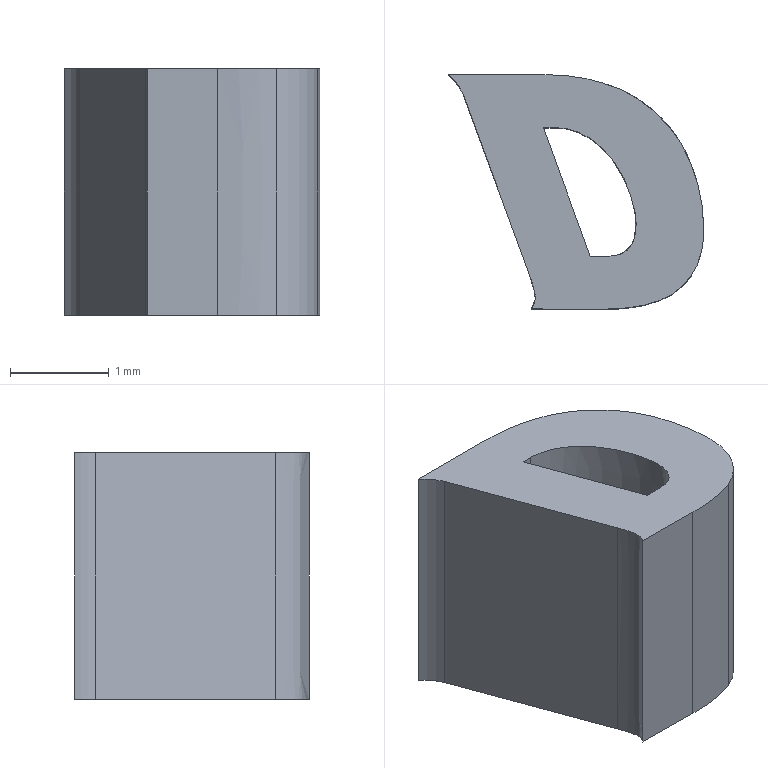Part | STEP file | lll_id1118_x_t | 1 solid | 17 faces | box 2.599 x 2.384 x 2.5 mm | volume 9.059 mm3 | plane 8 | other 6 | cylinder 3 | commonest cylinder face diameters 1.036 x1 1.35 x1 2.111 x1
STEP:
#1=CARTESIAN_POINT('',(392.289,-127.34,2.35));
#2=VERTEX_POINT('',#1);
#3=CARTESIAN_POINT('',(392.454,-127.34,2.35));
#4=VERTEX_POINT('',#3);
#5=CARTESIAN_POINT('',(392.289,-127.34,2.35));
#6=DIRECTION('',(1.,0.,0.));
#7=VECTOR('',#6,1.);
#8=LINE('',#5,#7);
#9=EDGE_CURVE('',#2,#4,#8,.T.);
#10=ORIENTED_EDGE('',*,*,#9,.T.);
#11=CARTESIAN_POINT('',(392.454,-127.34,-0.15));
#12=VERTEX_POINT('',#11);
#13=CARTESIAN_POINT('',(392.454,-127.34,-0.15));
#14=DIRECTION('',(0.,0.,1.));
#15=VECTOR('',#14,1.);
#16=LINE('',#13,#15);
#17=EDGE_CURVE('',#12,#4,#16,.T.);
#18=ORIENTED_EDGE('',*,*,#17,.F.);
#19=CARTESIAN_POINT('',(392.289,-127.34,-0.15));
#20=VERTEX_POINT('',#19);
#21=CARTESIAN_POINT('',(392.289,-127.34,-0.15));
#22=DIRECTION('',(1.,0.,0.));
#23=VECTOR('',#22,1.);
#24=LINE('',#21,#23);
#25=EDGE_CURVE('',#20,#12,#24,.T.);
#26=ORIENTED_EDGE('',*,*,#25,.F.);
#27=CARTESIAN_POINT('',(392.289,-127.34,-0.15));
#28=DIRECTION('',(0.,0.,1.));
#29=VECTOR('',#28,1.);
#30=LINE('',#27,#29);
#31=EDGE_CURVE('',#20,#2,#30,.T.);
#32=ORIENTED_EDGE('',*,*,#31,.T.);
#33=EDGE_LOOP('',(#10,#18,#26,#32));
#34=FACE_OUTER_BOUND('',#33,.T.);
#35=CARTESIAN_POINT('',(392.289,-127.34,-0.15));
#36=DIRECTION('',(0.,-1.,0.));
#37=DIRECTION('',(0.,0.,-1.));
#38=AXIS2_PLACEMENT_3D('',#35,#36,#37);
#39=PLANE('',#38);
#40=ADVANCED_FACE('',(#34),#39,.F.);
#41=CARTESIAN_POINT('',(392.629,-127.301,2.35));
#42=VERTEX_POINT('',#41);
#43=CARTESIAN_POINT('',(392.454,-127.34,2.35));
#44=CARTESIAN_POINT('',(392.485,-127.34,2.35));
#45=CARTESIAN_POINT('',(392.515,-127.337,2.35));
#46=CARTESIAN_POINT('',(392.574,-127.326,2.35));
#47=CARTESIAN_POINT('',(392.603,-127.316,2.35));
#48=CARTESIAN_POINT('',(392.629,-127.301,2.35));
#49=(BOUNDED_CURVE()B_SPLINE_CURVE(3,(#43,#44,#45,#46,#47,#48),.UNSPECIFIED.,.F.,.F.)B_SPLINE_CURVE_WITH_KNOTS((4,2,4),(0.,0.5014,1.),.UNSPECIFIED.)CURVE()GEOMETRIC_REPRESENTATION_ITEM()RATIONAL_B_SPLINE_CURVE((0.5011,0.4996,0.4996,0.4968,0.4968,0.5011))REPRESENTATION_ITEM(''));
#50=EDGE_CURVE('',#4,#42,#49,.T.);
#51=ORIENTED_EDGE('',*,*,#50,.T.);
#52=CARTESIAN_POINT('',(392.629,-127.301,-0.15));
#53=VERTEX_POINT('',#52);
#54=CARTESIAN_POINT('',(392.629,-127.301,-0.15));
#55=DIRECTION('',(0.,0.,1.));
#56=VECTOR('',#55,1.);
#57=LINE('',#54,#56);
#58=EDGE_CURVE('',#53,#42,#57,.T.);
#59=ORIENTED_EDGE('',*,*,#58,.F.);
#60=CARTESIAN_POINT('',(392.454,-127.34,-0.15));
#61=CARTESIAN_POINT('',(392.485,-127.34,-0.15));
#62=CARTESIAN_POINT('',(392.515,-127.337,-0.15));
#63=CARTESIAN_POINT('',(392.574,-127.326,-0.15));
#64=CARTESIAN_POINT('',(392.603,-127.316,-0.15));
#65=CARTESIAN_POINT('',(392.629,-127.301,-0.15));
#66=(BOUNDED_CURVE()B_SPLINE_CURVE(3,(#60,#61,#62,#63,#64,#65),.UNSPECIFIED.,.F.,.F.)B_SPLINE_CURVE_WITH_KNOTS((4,2,4),(0.,0.5014,1.),.UNSPECIFIED.)CURVE()GEOMETRIC_REPRESENTATION_ITEM()RATIONAL_B_SPLINE_CURVE((0.5011,0.4996,0.4996,0.4968,0.4968,0.5011))REPRESENTATION_ITEM(''));
#67=EDGE_CURVE('',#12,#53,#66,.T.);
#68=ORIENTED_EDGE('',*,*,#67,.F.);
#69=ORIENTED_EDGE('',*,*,#17,.T.);
#70=EDGE_LOOP('',(#51,#59,#68,#69));
#71=FACE_OUTER_BOUND('',#70,.T.);
#72=CARTESIAN_POINT('',(392.454,-127.34,-0.15));
#73=CARTESIAN_POINT('',(392.485,-127.34,-0.15));
#74=CARTESIAN_POINT('',(392.515,-127.337,-0.15));
#75=CARTESIAN_POINT('',(392.574,-127.326,-0.15));
#76=CARTESIAN_POINT('',(392.603,-127.316,-0.15));
#77=CARTESIAN_POINT('',(392.629,-127.301,-0.15));
#78=(BOUNDED_CURVE()B_SPLINE_CURVE(3,(#72,#73,#74,#75,#76,#77),.UNSPECIFIED.,.F.,.F.)B_SPLINE_CURVE_WITH_KNOTS((4,2,4),(0.,0.5014,1.),.UNSPECIFIED.)CURVE()GEOMETRIC_REPRESENTATION_ITEM()RATIONAL_B_SPLINE_CURVE((0.5011,0.4996,0.4996,0.4968,0.4968,0.5011))REPRESENTATION_ITEM(''));
#79=DIRECTION('',(0.,0.,1.));
#80=VECTOR('',#79,1.);
#81=SURFACE_OF_LINEAR_EXTRUSION('',#78,#80);
#82=ADVANCED_FACE('',(#71),#81,.F.);
#83=CARTESIAN_POINT('',(391.925,-126.033,2.35));
#84=VERTEX_POINT('',#83);
#85=CARTESIAN_POINT('',(392.629,-127.301,2.35));
#86=CARTESIAN_POINT('',(392.664,-127.281,2.35));
#87=CARTESIAN_POINT('',(392.693,-127.252,2.35));
#88=CARTESIAN_POINT('',(392.724,-127.194,2.35));
#89=CARTESIAN_POINT('',(392.733,-127.17,2.35));
#90=CARTESIAN_POINT('',(392.748,-127.112,2.35));
#91=CARTESIAN_POINT('',(392.753,-127.077,2.35));
#92=CARTESIAN_POINT('',(392.755,-127.012,2.35));
#93=CARTESIAN_POINT('',(392.754,-126.982,2.35));
#94=CARTESIAN_POINT('',(392.746,-126.903,2.35));
#95=CARTESIAN_POINT('',(392.737,-126.854,2.35));
#96=CARTESIAN_POINT('',(392.689,-126.67,2.35));
#97=CARTESIAN_POINT('',(392.635,-126.542,2.35));
#98=CARTESIAN_POINT('',(392.512,-126.348,2.35));
#99=CARTESIAN_POINT('',(392.454,-126.279,2.35));
#100=CARTESIAN_POINT('',(392.321,-126.158,2.35));
#101=CARTESIAN_POINT('',(392.244,-126.11,2.35));
#102=CARTESIAN_POINT('',(392.085,-126.047,2.35));
#103=CARTESIAN_POINT('',(392.006,-126.033,2.35));
#104=CARTESIAN_POINT('',(391.925,-126.033,2.35));
#105=(BOUNDED_CURVE()B_SPLINE_CURVE(3,(#85,#86,#87,#88,#89,#90,#91,#92,#93,#94,#95,#96,#97,#98,#99,#100,#101,#102,#103,#104),.UNSPECIFIED.,.F.,.F.)B_SPLINE_CURVE_WITH_KNOTS((4,2,2,2,2,2,2,2,2,4),(0.,0.07173,0.1159,0.1772,0.2294,0.3163,0.5576,0.7116,0.8649,1.),.UNSPECIFIED.)CURVE()GEOMETRIC_REPRESENTATION_ITEM()RATIONAL_B_SPLINE_CURVE((0.5011,0.4882,0.4882,0.4987,0.4987,0.499,0.499,0.5004,0.5004,0.5001,0.5001,0.497,0.497,0.4981,0.4981,0.4957,0.4957,0.4952,0.4952,0.5011))REPRESENTATION_ITEM(''));
#106=EDGE_CURVE('',#42,#84,#105,.T.);
#107=ORIENTED_EDGE('',*,*,#106,.T.);
#108=CARTESIAN_POINT('',(391.925,-126.033,-0.15));
#109=VERTEX_POINT('',#108);
#110=CARTESIAN_POINT('',(391.925,-126.033,-0.15));
#111=DIRECTION('',(0.,0.,1.));
#112=VECTOR('',#111,1.);
#113=LINE('',#110,#112);
#114=EDGE_CURVE('',#109,#84,#113,.T.);
#115=ORIENTED_EDGE('',*,*,#114,.F.);
#116=CARTESIAN_POINT('',(392.629,-127.301,-0.15));
#117=CARTESIAN_POINT('',(392.664,-127.281,-0.15));
#118=CARTESIAN_POINT('',(392.693,-127.252,-0.15));
#119=CARTESIAN_POINT('',(392.724,-127.194,-0.15));
#120=CARTESIAN_POINT('',(392.733,-127.17,-0.15));
#121=CARTESIAN_POINT('',(392.748,-127.112,-0.15));
#122=CARTESIAN_POINT('',(392.753,-127.077,-0.15));
#123=CARTESIAN_POINT('',(392.755,-127.012,-0.15));
#124=CARTESIAN_POINT('',(392.754,-126.982,-0.15));
#125=CARTESIAN_POINT('',(392.746,-126.903,-0.15));
#126=CARTESIAN_POINT('',(392.737,-126.854,-0.15));
#127=CARTESIAN_POINT('',(392.689,-126.67,-0.15));
#128=CARTESIAN_POINT('',(392.635,-126.542,-0.15));
#129=CARTESIAN_POINT('',(392.512,-126.348,-0.15));
#130=CARTESIAN_POINT('',(392.454,-126.279,-0.15));
#131=CARTESIAN_POINT('',(392.321,-126.158,-0.15));
#132=CARTESIAN_POINT('',(392.244,-126.11,-0.15));
#133=CARTESIAN_POINT('',(392.085,-126.047,-0.15));
#134=CARTESIAN_POINT('',(392.006,-126.033,-0.15));
#135=CARTESIAN_POINT('',(391.925,-126.033,-0.15));
#136=(BOUNDED_CURVE()B_SPLINE_CURVE(3,(#116,#117,#118,#119,#120,#121,#122,#123,#124,#125,#126,#127,#128,#129,#130,#131,#132,#133,#134,#135),.UNSPECIFIED.,.F.,.F.)B_SPLINE_CURVE_WITH_KNOTS((4,2,2,2,2,2,2,2,2,4),(0.,0.07173,0.1159,0.1772,0.2294,0.3163,0.5576,0.7116,0.8649,1.),.UNSPECIFIED.)CURVE()GEOMETRIC_REPRESENTATION_ITEM()RATIONAL_B_SPLINE_CURVE((0.5011,0.4882,0.4882,0.4987,0.4987,0.499,0.499,0.5004,0.5004,0.5001,0.5001,0.497,0.497,0.4981,0.4981,0.4957,0.4957,0.4952,0.4952,0.5011))REPRESENTATION_ITEM(''));
#137=EDGE_CURVE('',#53,#109,#136,.T.);
#138=ORIENTED_EDGE('',*,*,#137,.F.);
#139=ORIENTED_EDGE('',*,*,#58,.T.);
#140=EDGE_LOOP('',(#107,#115,#138,#139));
#141=FACE_OUTER_BOUND('',#140,.T.);
#142=CARTESIAN_POINT('',(392.629,-127.301,-0.15));
#143=CARTESIAN_POINT('',(392.664,-127.281,-0.15));
#144=CARTESIAN_POINT('',(392.693,-127.252,-0.15));
#145=CARTESIAN_POINT('',(392.724,-127.194,-0.15));
#146=CARTESIAN_POINT('',(392.733,-127.17,-0.15));
#147=CARTESIAN_POINT('',(392.748,-127.112,-0.15));
#148=CARTESIAN_POINT('',(392.753,-127.077,-0.15));
#149=CARTESIAN_POINT('',(392.755,-127.012,-0.15));
#150=CARTESIAN_POINT('',(392.754,-126.982,-0.15));
#151=CARTESIAN_POINT('',(392.746,-126.903,-0.15));
#152=CARTESIAN_POINT('',(392.737,-126.854,-0.15));
#153=CARTESIAN_POINT('',(392.689,-126.67,-0.15));
#154=CARTESIAN_POINT('',(392.635,-126.542,-0.15));
#155=CARTESIAN_POINT('',(392.512,-126.348,-0.15));
#156=CARTESIAN_POINT('',(392.454,-126.279,-0.15));
#157=CARTESIAN_POINT('',(392.321,-126.158,-0.15));
#158=CARTESIAN_POINT('',(392.244,-126.11,-0.15));
#159=CARTESIAN_POINT('',(392.085,-126.047,-0.15));
#160=CARTESIAN_POINT('',(392.006,-126.033,-0.15));
#161=CARTESIAN_POINT('',(391.925,-126.033,-0.15));
#162=(BOUNDED_CURVE()B_SPLINE_CURVE(3,(#142,#143,#144,#145,#146,#147,#148,#149,#150,#151,#152,#153,#154,#155,#156,#157,#158,#159,#160,#161),.UNSPECIFIED.,.F.,.F.)B_SPLINE_CURVE_WITH_KNOTS((4,2,2,2,2,2,2,2,2,4),(0.,0.07173,0.1159,0.1772,0.2294,0.3163,0.5576,0.7116,0.8649,1.),.UNSPECIFIED.)CURVE()GEOMETRIC_REPRESENTATION_ITEM()RATIONAL_B_SPLINE_CURVE((0.5011,0.4882,0.4882,0.4987,0.4987,0.499,0.499,0.5004,0.5004,0.5001,0.5001,0.497,0.497,0.4981,0.4981,0.4957,0.4957,0.4952,0.4952,0.5011))REPRESENTATION_ITEM(''));
#163=DIRECTION('',(0.,0.,1.));
#164=VECTOR('',#163,1.);
#165=SURFACE_OF_LINEAR_EXTRUSION('',#162,#164);
#166=ADVANCED_FACE('',(#141),#165,.F.);
#167=CARTESIAN_POINT('',(391.814,-126.033,2.35));
#168=VERTEX_POINT('',#167);
#169=CARTESIAN_POINT('',(391.925,-126.033,2.35));
#170=DIRECTION('',(-1.,0.,0.));
#171=VECTOR('',#170,1.);
#172=LINE('',#169,#171);
#173=EDGE_CURVE('',#84,#168,#172,.T.);
#174=ORIENTED_EDGE('',*,*,#173,.T.);
#175=CARTESIAN_POINT('',(391.814,-126.033,-0.15));
#176=VERTEX_POINT('',#175);
#177=CARTESIAN_POINT('',(391.814,-126.033,-0.15));
#178=DIRECTION('',(0.,0.,1.));
#179=VECTOR('',#178,1.);
#180=LINE('',#177,#179);
#181=EDGE_CURVE('',#176,#168,#180,.T.);
#182=ORIENTED_EDGE('',*,*,#181,.F.);
#183=CARTESIAN_POINT('',(391.925,-126.033,-0.15));
#184=DIRECTION('',(-1.,0.,0.));
#185=VECTOR('',#184,1.);
#186=LINE('',#183,#185);
#187=EDGE_CURVE('',#109,#176,#186,.T.);
#188=ORIENTED_EDGE('',*,*,#187,.F.);
#189=ORIENTED_EDGE('',*,*,#114,.T.);
#190=EDGE_LOOP('',(#174,#182,#188,#189));
#191=FACE_OUTER_BOUND('',#190,.T.);
#192=CARTESIAN_POINT('',(391.925,-126.033,-0.15));
#193=DIRECTION('',(0.,1.,0.));
#194=DIRECTION('',(0.,0.,1.));
#195=AXIS2_PLACEMENT_3D('',#192,#193,#194);
#196=PLANE('',#195);
#197=ADVANCED_FACE('',(#191),#196,.F.);
#198=CARTESIAN_POINT('',(391.787,-125.492,2.35));
#199=VERTEX_POINT('',#198);
#200=CARTESIAN_POINT('',(392.416,-125.579,2.35));
#201=VERTEX_POINT('',#200);
#202=CARTESIAN_POINT('',(391.787,-125.492,2.35));
#203=CARTESIAN_POINT('',(391.894,-125.492,2.35));
#204=CARTESIAN_POINT('',(392.,-125.499,2.35));
#205=CARTESIAN_POINT('',(392.211,-125.526,2.35));
#206=CARTESIAN_POINT('',(392.315,-125.548,2.35));
#207=CARTESIAN_POINT('',(392.416,-125.579,2.35));
#208=(BOUNDED_CURVE()B_SPLINE_CURVE(3,(#202,#203,#204,#205,#206,#207),.UNSPECIFIED.,.F.,.F.)B_SPLINE_CURVE_WITH_KNOTS((4,2,4),(0.,0.5009,1.),.UNSPECIFIED.)CURVE()GEOMETRIC_REPRESENTATION_ITEM()RATIONAL_B_SPLINE_CURVE((0.5005,0.4998,0.4998,0.4993,0.4993,0.5005))REPRESENTATION_ITEM(''));
#209=EDGE_CURVE('',#199,#201,#208,.T.);
#210=ORIENTED_EDGE('',*,*,#209,.T.);
#211=CARTESIAN_POINT('',(392.416,-125.579,-0.15));
#212=VERTEX_POINT('',#211);
#213=CARTESIAN_POINT('',(392.416,-125.579,-0.15));
#214=DIRECTION('',(0.,0.,1.));
#215=VECTOR('',#214,1.);
#216=LINE('',#213,#215);
#217=EDGE_CURVE('',#212,#201,#216,.T.);
#218=ORIENTED_EDGE('',*,*,#217,.F.);
#219=CARTESIAN_POINT('',(391.787,-125.492,-0.15));
#220=VERTEX_POINT('',#219);
#221=CARTESIAN_POINT('',(391.787,-125.492,-0.15));
#222=CARTESIAN_POINT('',(391.894,-125.492,-0.15));
#223=CARTESIAN_POINT('',(392.,-125.499,-0.15));
#224=CARTESIAN_POINT('',(392.211,-125.526,-0.15));
#225=CARTESIAN_POINT('',(392.315,-125.548,-0.15));
#226=CARTESIAN_POINT('',(392.416,-125.579,-0.15));
#227=(BOUNDED_CURVE()B_SPLINE_CURVE(3,(#221,#222,#223,#224,#225,#226),.UNSPECIFIED.,.F.,.F.)B_SPLINE_CURVE_WITH_KNOTS((4,2,4),(0.,0.5009,1.),.UNSPECIFIED.)CURVE()GEOMETRIC_REPRESENTATION_ITEM()RATIONAL_B_SPLINE_CURVE((0.5005,0.4998,0.4998,0.4993,0.4993,0.5005))REPRESENTATION_ITEM(''));
#228=EDGE_CURVE('',#220,#212,#227,.T.);
#229=ORIENTED_EDGE('',*,*,#228,.F.);
#230=CARTESIAN_POINT('',(391.787,-125.492,-0.15));
#231=DIRECTION('',(0.,0.,1.));
#232=VECTOR('',#231,1.);
#233=LINE('',#230,#232);
#234=EDGE_CURVE('',#220,#199,#233,.T.);
#235=ORIENTED_EDGE('',*,*,#234,.T.);
#236=EDGE_LOOP('',(#210,#218,#229,#235));
#237=FACE_OUTER_BOUND('',#236,.T.);
#238=CARTESIAN_POINT('',(391.787,-125.492,-0.15));
#239=CARTESIAN_POINT('',(391.894,-125.492,-0.15));
#240=CARTESIAN_POINT('',(392.,-125.499,-0.15));
#241=CARTESIAN_POINT('',(392.211,-125.526,-0.15));
#242=CARTESIAN_POINT('',(392.315,-125.548,-0.15));
#243=CARTESIAN_POINT('',(392.416,-125.579,-0.15));
#244=(BOUNDED_CURVE()B_SPLINE_CURVE(3,(#238,#239,#240,#241,#242,#243),.UNSPECIFIED.,.F.,.F.)B_SPLINE_CURVE_WITH_KNOTS((4,2,4),(0.,0.5009,1.),.UNSPECIFIED.)CURVE()GEOMETRIC_REPRESENTATION_ITEM()RATIONAL_B_SPLINE_CURVE((0.5005,0.4998,0.4998,0.4993,0.4993,0.5005))REPRESENTATION_ITEM(''));
#245=DIRECTION('',(0.,0.,1.));
#246=VECTOR('',#245,1.);
#247=SURFACE_OF_LINEAR_EXTRUSION('',#244,#246);
#248=ADVANCED_FACE('',(#237),#247,.F.);
#249=CARTESIAN_POINT('',(393.44,-127.036,2.35));
#250=VERTEX_POINT('',#249);
#251=CARTESIAN_POINT('',(392.416,-125.579,2.35));
#252=CARTESIAN_POINT('',(392.794,-125.689,2.35));
#253=CARTESIAN_POINT('',(393.095,-125.944,2.35));
#254=CARTESIAN_POINT('',(393.303,-126.374,2.35));
#255=CARTESIAN_POINT('',(393.334,-126.453,2.35));
#256=CARTESIAN_POINT('',(393.408,-126.698,2.35));
#257=CARTESIAN_POINT('',(393.436,-126.866,2.35));
#258=CARTESIAN_POINT('',(393.44,-127.036,2.35));
#259=(BOUNDED_CURVE()B_SPLINE_CURVE(3,(#251,#252,#253,#254,#255,#256,#257,#258),.UNSPECIFIED.,.F.,.F.)B_SPLINE_CURVE_WITH_KNOTS((4,2,2,4),(0.,0.6081,0.739,1.),.UNSPECIFIED.)CURVE()GEOMETRIC_REPRESENTATION_ITEM()RATIONAL_B_SPLINE_CURVE((0.5005,0.4717,0.4717,0.4994,0.4994,0.4973,0.4973,0.5005))REPRESENTATION_ITEM(''));
#260=EDGE_CURVE('',#201,#250,#259,.T.);
#261=ORIENTED_EDGE('',*,*,#260,.T.);
#262=CARTESIAN_POINT('',(393.44,-127.036,-0.15));
#263=VERTEX_POINT('',#262);
#264=CARTESIAN_POINT('',(393.44,-127.036,-0.15));
#265=DIRECTION('',(0.,0.,1.));
#266=VECTOR('',#265,1.);
#267=LINE('',#264,#266);
#268=EDGE_CURVE('',#263,#250,#267,.T.);
#269=ORIENTED_EDGE('',*,*,#268,.F.);
#270=CARTESIAN_POINT('',(392.416,-125.579,-0.15));
#271=CARTESIAN_POINT('',(392.794,-125.689,-0.15));
#272=CARTESIAN_POINT('',(393.095,-125.944,-0.15));
#273=CARTESIAN_POINT('',(393.303,-126.374,-0.15));
#274=CARTESIAN_POINT('',(393.334,-126.453,-0.15));
#275=CARTESIAN_POINT('',(393.408,-126.698,-0.15));
#276=CARTESIAN_POINT('',(393.436,-126.866,-0.15));
#277=CARTESIAN_POINT('',(393.44,-127.036,-0.15));
#278=(BOUNDED_CURVE()B_SPLINE_CURVE(3,(#270,#271,#272,#273,#274,#275,#276,#277),.UNSPECIFIED.,.F.,.F.)B_SPLINE_CURVE_WITH_KNOTS((4,2,2,4),(0.,0.6081,0.739,1.),.UNSPECIFIED.)CURVE()GEOMETRIC_REPRESENTATION_ITEM()RATIONAL_B_SPLINE_CURVE((0.5005,0.4717,0.4717,0.4994,0.4994,0.4973,0.4973,0.5005))REPRESENTATION_ITEM(''));
#279=EDGE_CURVE('',#212,#263,#278,.T.);
#280=ORIENTED_EDGE('',*,*,#279,.F.);
#281=ORIENTED_EDGE('',*,*,#217,.T.);
#282=EDGE_LOOP('',(#261,#269,#280,#281));
#283=FACE_OUTER_BOUND('',#282,.T.);
#284=CARTESIAN_POINT('',(392.416,-125.579,-0.15));
#285=CARTESIAN_POINT('',(392.794,-125.689,-0.15));
#286=CARTESIAN_POINT('',(393.095,-125.944,-0.15));
#287=CARTESIAN_POINT('',(393.303,-126.374,-0.15));
#288=CARTESIAN_POINT('',(393.334,-126.453,-0.15));
#289=CARTESIAN_POINT('',(393.408,-126.698,-0.15));
#290=CARTESIAN_POINT('',(393.436,-126.866,-0.15));
#291=CARTESIAN_POINT('',(393.44,-127.036,-0.15));
#292=(BOUNDED_CURVE()B_SPLINE_CURVE(3,(#284,#285,#286,#287,#288,#289,#290,#291),.UNSPECIFIED.,.F.,.F.)B_SPLINE_CURVE_WITH_KNOTS((4,2,2,4),(0.,0.6081,0.739,1.),.UNSPECIFIED.)CURVE()GEOMETRIC_REPRESENTATION_ITEM()RATIONAL_B_SPLINE_CURVE((0.5005,0.4717,0.4717,0.4994,0.4994,0.4973,0.4973,0.5005))REPRESENTATION_ITEM(''));
#293=DIRECTION('',(0.,0.,1.));
#294=VECTOR('',#293,1.);
#295=SURFACE_OF_LINEAR_EXTRUSION('',#292,#294);
#296=ADVANCED_FACE('',(#283),#295,.F.);
#297=CARTESIAN_POINT('',(393.418,-127.29,2.35));
#298=VERTEX_POINT('',#297);
#299=CARTESIAN_POINT('',(392.386,-127.071,2.35));
#300=DIRECTION('',(0.,0.,-1.));
#301=DIRECTION('',(1.,0.,0.));
#302=AXIS2_PLACEMENT_3D('',#299,#300,#301);
#303=CIRCLE('',#302,1.055);
#304=EDGE_CURVE('',#250,#298,#303,.T.);
#305=ORIENTED_EDGE('',*,*,#304,.T.);
#306=CARTESIAN_POINT('',(393.418,-127.29,-0.15));
#307=VERTEX_POINT('',#306);
#308=CARTESIAN_POINT('',(393.418,-127.29,-0.15));
#309=DIRECTION('',(0.,0.,1.));
#310=VECTOR('',#309,1.);
#311=LINE('',#308,#310);
#312=EDGE_CURVE('',#307,#298,#311,.T.);
#313=ORIENTED_EDGE('',*,*,#312,.F.);
#314=CARTESIAN_POINT('',(392.386,-127.071,-0.15));
#315=DIRECTION('',(0.,0.,-1.));
#316=DIRECTION('',(1.,0.,0.));
#317=AXIS2_PLACEMENT_3D('',#314,#315,#316);
#318=CIRCLE('',#317,1.055);
#319=EDGE_CURVE('',#263,#307,#318,.T.);
#320=ORIENTED_EDGE('',*,*,#319,.F.);
#321=ORIENTED_EDGE('',*,*,#268,.T.);
#322=EDGE_LOOP('',(#305,#313,#320,#321));
#323=FACE_OUTER_BOUND('',#322,.T.);
#324=CARTESIAN_POINT('',(392.386,-127.071,-0.15));
#325=DIRECTION('',(0.,0.,1.));
#326=DIRECTION('',(1.,0.,0.));
#327=AXIS2_PLACEMENT_3D('',#324,#325,#326);
#328=CYLINDRICAL_SURFACE('',#327,1.055);
#329=ADVANCED_FACE('',(#323),#328,.T.);
#330=CARTESIAN_POINT('',(393.004,-127.784,2.35));
#331=VERTEX_POINT('',#330);
#332=CARTESIAN_POINT('',(392.756,-127.156,2.35));
#333=DIRECTION('',(0.,0.,-1.));
#334=DIRECTION('',(1.,0.,0.));
#335=AXIS2_PLACEMENT_3D('',#332,#333,#334);
#336=CIRCLE('',#335,0.6752);
#337=EDGE_CURVE('',#298,#331,#336,.T.);
#338=ORIENTED_EDGE('',*,*,#337,.T.);
#339=CARTESIAN_POINT('',(393.004,-127.784,-0.15));
#340=VERTEX_POINT('',#339);
#341=CARTESIAN_POINT('',(393.004,-127.784,-0.15));
#342=DIRECTION('',(0.,0.,1.));
#343=VECTOR('',#342,1.);
#344=LINE('',#341,#343);
#345=EDGE_CURVE('',#340,#331,#344,.T.);
#346=ORIENTED_EDGE('',*,*,#345,.F.);
#347=CARTESIAN_POINT('',(392.756,-127.156,-0.15));
#348=DIRECTION('',(0.,0.,-1.));
#349=DIRECTION('',(1.,0.,0.));
#350=AXIS2_PLACEMENT_3D('',#347,#348,#349);
#351=CIRCLE('',#350,0.6752);
#352=EDGE_CURVE('',#307,#340,#351,.T.);
#353=ORIENTED_EDGE('',*,*,#352,.F.);
#354=ORIENTED_EDGE('',*,*,#312,.T.);
#355=EDGE_LOOP('',(#338,#346,#353,#354));
#356=FACE_OUTER_BOUND('',#355,.T.);
#357=CARTESIAN_POINT('',(392.756,-127.156,-0.15));
#358=DIRECTION('',(0.,0.,1.));
#359=DIRECTION('',(1.,0.,0.));
#360=AXIS2_PLACEMENT_3D('',#357,#358,#359);
#361=CYLINDRICAL_SURFACE('',#360,0.6752);
#362=ADVANCED_FACE('',(#356),#361,.T.);
#363=CARTESIAN_POINT('',(392.408,-127.876,2.35));
#364=VERTEX_POINT('',#363);
#365=CARTESIAN_POINT('',(393.004,-127.784,2.35));
#366=CARTESIAN_POINT('',(392.955,-127.804,2.35));
#367=CARTESIAN_POINT('',(392.904,-127.82,2.35));
#368=CARTESIAN_POINT('',(392.789,-127.846,2.35));
#369=CARTESIAN_POINT('',(392.727,-127.857,2.35));
#370=CARTESIAN_POINT('',(392.578,-127.873,2.35));
#371=CARTESIAN_POINT('',(392.493,-127.878,2.35));
#372=CARTESIAN_POINT('',(392.408,-127.876,2.35));
#373=(BOUNDED_CURVE()B_SPLINE_CURVE(3,(#365,#366,#367,#368,#369,#370,#371,#372),.UNSPECIFIED.,.F.,.F.)B_SPLINE_CURVE_WITH_KNOTS((4,2,2,4),(0.,0.2638,0.5793,1.),.UNSPECIFIED.)CURVE()GEOMETRIC_REPRESENTATION_ITEM()RATIONAL_B_SPLINE_CURVE((0.5005,0.4994,0.4994,0.4999,0.4999,0.4999,0.4999,0.5005))REPRESENTATION_ITEM(''));
#374=EDGE_CURVE('',#331,#364,#373,.T.);
#375=ORIENTED_EDGE('',*,*,#374,.T.);
#376=CARTESIAN_POINT('',(392.408,-127.876,-0.15));
#377=VERTEX_POINT('',#376);
#378=CARTESIAN_POINT('',(392.408,-127.876,-0.15));
#379=DIRECTION('',(0.,0.,1.));
#380=VECTOR('',#379,1.);
#381=LINE('',#378,#380);
#382=EDGE_CURVE('',#377,#364,#381,.T.);
#383=ORIENTED_EDGE('',*,*,#382,.F.);
#384=CARTESIAN_POINT('',(393.004,-127.784,-0.15));
#385=CARTESIAN_POINT('',(392.955,-127.804,-0.15));
#386=CARTESIAN_POINT('',(392.904,-127.82,-0.15));
#387=CARTESIAN_POINT('',(392.789,-127.846,-0.15));
#388=CARTESIAN_POINT('',(392.727,-127.857,-0.15));
#389=CARTESIAN_POINT('',(392.578,-127.873,-0.15));
#390=CARTESIAN_POINT('',(392.493,-127.878,-0.15));
#391=CARTESIAN_POINT('',(392.408,-127.876,-0.15));
#392=(BOUNDED_CURVE()B_SPLINE_CURVE(3,(#384,#385,#386,#387,#388,#389,#390,#391),.UNSPECIFIED.,.F.,.F.)B_SPLINE_CURVE_WITH_KNOTS((4,2,2,4),(0.,0.2638,0.5793,1.),.UNSPECIFIED.)CURVE()GEOMETRIC_REPRESENTATION_ITEM()RATIONAL_B_SPLINE_CURVE((0.5005,0.4994,0.4994,0.4999,0.4999,0.4999,0.4999,0.5005))REPRESENTATION_ITEM(''));
#393=EDGE_CURVE('',#340,#377,#392,.T.);
#394=ORIENTED_EDGE('',*,*,#393,.F.);
#395=ORIENTED_EDGE('',*,*,#345,.T.);
#396=EDGE_LOOP('',(#375,#383,#394,#395));
#397=FACE_OUTER_BOUND('',#396,.T.);
#398=CARTESIAN_POINT('',(393.004,-127.784,-0.15));
#399=CARTESIAN_POINT('',(392.955,-127.804,-0.15));
#400=CARTESIAN_POINT('',(392.904,-127.82,-0.15));
#401=CARTESIAN_POINT('',(392.789,-127.846,-0.15));
#402=CARTESIAN_POINT('',(392.727,-127.857,-0.15));
#403=CARTESIAN_POINT('',(392.578,-127.873,-0.15));
#404=CARTESIAN_POINT('',(392.493,-127.878,-0.15));
#405=CARTESIAN_POINT('',(392.408,-127.876,-0.15));
#406=(BOUNDED_CURVE()B_SPLINE_CURVE(3,(#398,#399,#400,#401,#402,#403,#404,#405),.UNSPECIFIED.,.F.,.F.)B_SPLINE_CURVE_WITH_KNOTS((4,2,2,4),(0.,0.2638,0.5793,1.),.UNSPECIFIED.)CURVE()GEOMETRIC_REPRESENTATION_ITEM()RATIONAL_B_SPLINE_CURVE((0.5005,0.4994,0.4994,0.4999,0.4999,0.4999,0.4999,0.5005))REPRESENTATION_ITEM(''));
#407=DIRECTION('',(0.,0.,1.));
#408=VECTOR('',#407,1.);
#409=SURFACE_OF_LINEAR_EXTRUSION('',#406,#408);
#410=ADVANCED_FACE('',(#397),#409,.F.);
#411=CARTESIAN_POINT('',(391.691,-127.874,2.35));
#412=VERTEX_POINT('',#411);
#413=CARTESIAN_POINT('',(392.408,-127.876,2.35));
#414=DIRECTION('',(-1.,0.,0.));
#415=VECTOR('',#414,1.);
#416=LINE('',#413,#415);
#417=EDGE_CURVE('',#364,#412,#416,.T.);
#418=ORIENTED_EDGE('',*,*,#417,.T.);
#419=CARTESIAN_POINT('',(391.691,-127.874,-0.15));
#420=VERTEX_POINT('',#419);
#421=CARTESIAN_POINT('',(391.686,-127.876,-0.15));
#422=DIRECTION('',(0.,0.,1.));
#423=VECTOR('',#422,1.);
#424=LINE('',#421,#423);
#425=EDGE_CURVE('',#420,#412,#424,.T.);
#426=ORIENTED_EDGE('',*,*,#425,.F.);
#427=CARTESIAN_POINT('',(392.408,-127.876,-0.15));
#428=DIRECTION('',(-1.,0.,0.));
#429=VECTOR('',#428,1.);
#430=LINE('',#427,#429);
#431=EDGE_CURVE('',#377,#420,#430,.T.);
#432=ORIENTED_EDGE('',*,*,#431,.F.);
#433=ORIENTED_EDGE('',*,*,#382,.T.);
#434=EDGE_LOOP('',(#418,#426,#432,#433));
#435=FACE_OUTER_BOUND('',#434,.T.);
#436=CARTESIAN_POINT('',(392.408,-127.876,-0.15));
#437=DIRECTION('',(0.,1.,0.));
#438=DIRECTION('',(0.,0.,1.));
#439=AXIS2_PLACEMENT_3D('',#436,#437,#438);
#440=PLANE('',#439);
#441=ADVANCED_FACE('',(#435),#440,.F.);
#442=CARTESIAN_POINT('',(391.674,-127.533,2.35));
#443=VERTEX_POINT('',#442);
#444=CARTESIAN_POINT('',(391.691,-127.871,2.35));
#445=CARTESIAN_POINT('',(391.713,-127.845,2.35));
#446=CARTESIAN_POINT('',(391.726,-127.814,2.35));
#447=CARTESIAN_POINT('',(391.73,-127.767,2.35));
#448=CARTESIAN_POINT('',(391.73,-127.754,2.35));
#449=CARTESIAN_POINT('',(391.729,-127.732,2.35));
#450=CARTESIAN_POINT('',(391.728,-127.723,2.35));
#451=CARTESIAN_POINT('',(391.724,-127.703,2.35));
#452=CARTESIAN_POINT('',(391.722,-127.692,2.35));
#453=CARTESIAN_POINT('',(391.717,-127.671,2.35));
#454=CARTESIAN_POINT('',(391.714,-127.66,2.35));
#455=CARTESIAN_POINT('',(391.704,-127.624,2.35));
#456=CARTESIAN_POINT('',(391.697,-127.599,2.35));
#457=CARTESIAN_POINT('',(391.684,-127.561,2.35));
#458=CARTESIAN_POINT('',(391.679,-127.547,2.35));
#459=CARTESIAN_POINT('',(391.674,-127.533,2.35));
#460=(BOUNDED_CURVE()B_SPLINE_CURVE(3,(#444,#445,#446,#447,#448,#449,#450,#451,#452,#453,#454,#455,#456,#457,#458,#459),.UNSPECIFIED.,.F.,.F.)B_SPLINE_CURVE_WITH_KNOTS((4,2,2,2,2,2,2,4),(0.,0.2854,0.3944,0.4719,0.5652,0.6585,0.8758,1.),.UNSPECIFIED.)CURVE()GEOMETRIC_REPRESENTATION_ITEM()RATIONAL_B_SPLINE_CURVE((0.5124,0.4959,0.4959,0.5111,0.5111,0.5121,0.5121,0.5122,0.5122,0.5123,0.5123,0.5123,0.5123,0.5123,0.5123,0.5124))REPRESENTATION_ITEM(''));
#461=EDGE_CURVE('',#412,#443,#460,.T.);
#462=ORIENTED_EDGE('',*,*,#461,.T.);
#463=CARTESIAN_POINT('',(391.674,-127.533,-0.15));
#464=VERTEX_POINT('',#463);
#465=CARTESIAN_POINT('',(391.674,-127.533,-0.15));
#466=DIRECTION('',(0.,0.,1.));
#467=VECTOR('',#466,1.);
#468=LINE('',#465,#467);
#469=EDGE_CURVE('',#464,#443,#468,.T.);
#470=ORIENTED_EDGE('',*,*,#469,.F.);
#471=CARTESIAN_POINT('',(391.688,-127.874,-0.15));
#472=CARTESIAN_POINT('',(391.689,-127.873,-0.15));
#473=CARTESIAN_POINT('',(391.69,-127.872,-0.15));
#474=CARTESIAN_POINT('',(391.713,-127.845,-0.15));
#475=CARTESIAN_POINT('',(391.726,-127.814,-0.15));
#476=CARTESIAN_POINT('',(391.73,-127.767,-0.15));
#477=CARTESIAN_POINT('',(391.73,-127.754,-0.15));
#478=CARTESIAN_POINT('',(391.729,-127.732,-0.15));
#479=CARTESIAN_POINT('',(391.728,-127.723,-0.15));
#480=CARTESIAN_POINT('',(391.724,-127.703,-0.15));
#481=CARTESIAN_POINT('',(391.722,-127.692,-0.15));
#482=CARTESIAN_POINT('',(391.717,-127.671,-0.15));
#483=CARTESIAN_POINT('',(391.714,-127.66,-0.15));
#484=CARTESIAN_POINT('',(391.704,-127.624,-0.15));
#485=CARTESIAN_POINT('',(391.697,-127.599,-0.15));
#486=CARTESIAN_POINT('',(391.684,-127.561,-0.15));
#487=CARTESIAN_POINT('',(391.679,-127.547,-0.15));
#488=CARTESIAN_POINT('',(391.674,-127.533,-0.15));
#489=(BOUNDED_CURVE()B_SPLINE_CURVE(3,(#471,#472,#473,#474,#475,#476,#477,#478,#479,#480,#481,#482,#483,#484,#485,#486,#487,#488),.UNSPECIFIED.,.F.,.F.)B_SPLINE_CURVE_WITH_KNOTS((4,2,2,2,2,2,2,2,4),(0.,0.009901,0.2925,0.4004,0.4772,0.5695,0.6619,0.877,1.),.UNSPECIFIED.)CURVE()GEOMETRIC_REPRESENTATION_ITEM()RATIONAL_B_SPLINE_CURVE((0.5124,0.5124,0.5124,0.4959,0.4959,0.5111,0.5111,0.5121,0.5121,0.5122,0.5122,0.5123,0.5123,0.5123,0.5123,0.5123,0.5123,0.5124))REPRESENTATION_ITEM(''));
#490=EDGE_CURVE('',#420,#464,#489,.T.);
#491=ORIENTED_EDGE('',*,*,#490,.F.);
#492=ORIENTED_EDGE('',*,*,#425,.T.);
#493=EDGE_LOOP('',(#462,#470,#491,#492));
#494=FACE_OUTER_BOUND('',#493,.T.);
#495=CARTESIAN_POINT('',(391.686,-127.876,-0.15));
#496=CARTESIAN_POINT('',(391.687,-127.875,-0.15));
#497=CARTESIAN_POINT('',(391.688,-127.874,-0.15));
#498=CARTESIAN_POINT('',(391.689,-127.873,-0.15));
#499=CARTESIAN_POINT('',(391.69,-127.872,-0.15));
#500=CARTESIAN_POINT('',(391.713,-127.845,-0.15));
#501=CARTESIAN_POINT('',(391.726,-127.814,-0.15));
#502=CARTESIAN_POINT('',(391.73,-127.767,-0.15));
#503=CARTESIAN_POINT('',(391.73,-127.754,-0.15));
#504=CARTESIAN_POINT('',(391.729,-127.732,-0.15));
#505=CARTESIAN_POINT('',(391.728,-127.723,-0.15));
#506=CARTESIAN_POINT('',(391.724,-127.703,-0.15));
#507=CARTESIAN_POINT('',(391.722,-127.692,-0.15));
#508=CARTESIAN_POINT('',(391.717,-127.671,-0.15));
#509=CARTESIAN_POINT('',(391.714,-127.66,-0.15));
#510=CARTESIAN_POINT('',(391.704,-127.624,-0.15));
#511=CARTESIAN_POINT('',(391.697,-127.599,-0.15));
#512=CARTESIAN_POINT('',(391.684,-127.561,-0.15));
#513=CARTESIAN_POINT('',(391.679,-127.547,-0.15));
#514=CARTESIAN_POINT('',(391.674,-127.533,-0.15));
#515=(BOUNDED_CURVE()B_SPLINE_CURVE(3,(#495,#496,#497,#498,#499,#500,#501,#502,#503,#504,#505,#506,#507,#508,#509,#510,#511,#512,#513,#514),.UNSPECIFIED.,.F.,.F.)B_SPLINE_CURVE_WITH_KNOTS((4,2,2,2,2,2,2,2,2,4),(0.,0.01075,0.02055,0.3001,0.4069,0.4828,0.5741,0.6655,0.8784,1.),.UNSPECIFIED.)CURVE()GEOMETRIC_REPRESENTATION_ITEM()RATIONAL_B_SPLINE_CURVE((0.5124,0.5124,0.5124,0.5124,0.5124,0.4959,0.4959,0.5111,0.5111,0.5121,0.5121,0.5122,0.5122,0.5123,0.5123,0.5123,0.5123,0.5123,0.5123,0.5124))REPRESENTATION_ITEM(''));
#516=DIRECTION('',(0.,0.,1.));
#517=VECTOR('',#516,1.);
#518=SURFACE_OF_LINEAR_EXTRUSION('',#515,#517);
#519=ADVANCED_FACE('',(#494),#518,.F.);
#520=CARTESIAN_POINT('',(391.005,-125.708,2.35));
#521=VERTEX_POINT('',#520);
#522=CARTESIAN_POINT('',(391.674,-127.533,2.35));
#523=DIRECTION('',(-0.3441,0.9389,0.));
#524=VECTOR('',#523,1.);
#525=LINE('',#522,#524);
#526=EDGE_CURVE('',#443,#521,#525,.T.);
#527=ORIENTED_EDGE('',*,*,#526,.T.);
#528=CARTESIAN_POINT('',(391.005,-125.708,-0.15));
#529=VERTEX_POINT('',#528);
#530=CARTESIAN_POINT('',(391.005,-125.708,-0.15));
#531=DIRECTION('',(0.,0.,1.));
#532=VECTOR('',#531,1.);
#533=LINE('',#530,#532);
#534=EDGE_CURVE('',#529,#521,#533,.T.);
#535=ORIENTED_EDGE('',*,*,#534,.F.);
#536=CARTESIAN_POINT('',(391.674,-127.533,-0.15));
#537=DIRECTION('',(-0.3441,0.9389,0.));
#538=VECTOR('',#537,1.);
#539=LINE('',#536,#538);
#540=EDGE_CURVE('',#464,#529,#539,.T.);
#541=ORIENTED_EDGE('',*,*,#540,.F.);
#542=ORIENTED_EDGE('',*,*,#469,.T.);
#543=EDGE_LOOP('',(#527,#535,#541,#542));
#544=FACE_OUTER_BOUND('',#543,.T.);
#545=CARTESIAN_POINT('',(391.674,-127.533,-0.15));
#546=DIRECTION('',(0.9389,0.3441,0.));
#547=DIRECTION('',(0.3441,-0.9389,0.));
#548=AXIS2_PLACEMENT_3D('',#545,#546,#547);
#549=PLANE('',#548);
#550=ADVANCED_FACE('',(#544),#549,.F.);
#551=CARTESIAN_POINT('',(390.848,-125.495,2.35));
#552=VERTEX_POINT('',#551);
#553=CARTESIAN_POINT('',(390.524,-125.902,2.35));
#554=DIRECTION('',(0.,0.,1.));
#555=DIRECTION('',(-1.,0.,0.));
#556=AXIS2_PLACEMENT_3D('',#553,#554,#555);
#557=CIRCLE('',#556,0.518);
#558=EDGE_CURVE('',#521,#552,#557,.T.);
#559=ORIENTED_EDGE('',*,*,#558,.T.);
#560=CARTESIAN_POINT('',(390.848,-125.495,-0.15));
#561=VERTEX_POINT('',#560);
#562=CARTESIAN_POINT('',(390.842,-125.492,-0.15));
#563=DIRECTION('',(0.,0.,1.));
#564=VECTOR('',#563,1.);
#565=LINE('',#562,#564);
#566=EDGE_CURVE('',#561,#552,#565,.T.);
#567=ORIENTED_EDGE('',*,*,#566,.F.);
#568=CARTESIAN_POINT('',(390.524,-125.902,-0.15));
#569=DIRECTION('',(0.,0.,1.));
#570=DIRECTION('',(-1.,0.,0.));
#571=AXIS2_PLACEMENT_3D('',#568,#569,#570);
#572=CIRCLE('',#571,0.518);
#573=EDGE_CURVE('',#529,#561,#572,.T.);
#574=ORIENTED_EDGE('',*,*,#573,.F.);
#575=ORIENTED_EDGE('',*,*,#534,.T.);
#576=EDGE_LOOP('',(#559,#567,#574,#575));
#577=FACE_OUTER_BOUND('',#576,.T.);
#578=CARTESIAN_POINT('',(390.524,-125.902,-0.15));
#579=DIRECTION('',(0.,0.,1.));
#580=DIRECTION('',(1.,0.,0.));
#581=AXIS2_PLACEMENT_3D('',#578,#579,#580);
#582=CYLINDRICAL_SURFACE('',#581,0.518);
#583=ADVANCED_FACE('',(#577),#582,.F.);
#584=CARTESIAN_POINT('',(390.848,-125.492,2.35));
#585=DIRECTION('',(1.,0.,0.));
#586=VECTOR('',#585,1.);
#587=LINE('',#584,#586);
#588=EDGE_CURVE('',#552,#199,#587,.T.);
#589=ORIENTED_EDGE('',*,*,#588,.T.);
#590=ORIENTED_EDGE('',*,*,#234,.F.);
#591=CARTESIAN_POINT('',(390.848,-125.492,-0.15));
#592=DIRECTION('',(1.,0.,0.));
#593=VECTOR('',#592,1.);
#594=LINE('',#591,#593);
#595=EDGE_CURVE('',#561,#220,#594,.T.);
#596=ORIENTED_EDGE('',*,*,#595,.F.);
#597=ORIENTED_EDGE('',*,*,#566,.T.);
#598=EDGE_LOOP('',(#589,#590,#596,#597));
#599=FACE_OUTER_BOUND('',#598,.T.);
#600=CARTESIAN_POINT('',(390.848,-125.492,-0.15));
#601=DIRECTION('',(0.,-1.,0.));
#602=DIRECTION('',(0.,0.,-1.));
#603=AXIS2_PLACEMENT_3D('',#600,#601,#602);
#604=PLANE('',#603);
#605=ADVANCED_FACE('',(#599),#604,.F.);
#606=CARTESIAN_POINT('',(391.814,-126.033,2.35));
#607=DIRECTION('',(0.3419,-0.9397,0.));
#608=VECTOR('',#607,1.);
#609=LINE('',#606,#608);
#610=EDGE_CURVE('',#168,#2,#609,.T.);
#611=ORIENTED_EDGE('',*,*,#610,.T.);
#612=ORIENTED_EDGE('',*,*,#31,.F.);
#613=CARTESIAN_POINT('',(391.814,-126.033,-0.15));
#614=DIRECTION('',(0.3419,-0.9397,0.));
#615=VECTOR('',#614,1.);
#616=LINE('',#613,#615);
#617=EDGE_CURVE('',#176,#20,#616,.T.);
#618=ORIENTED_EDGE('',*,*,#617,.F.);
#619=ORIENTED_EDGE('',*,*,#181,.T.);
#620=EDGE_LOOP('',(#611,#612,#618,#619));
#621=FACE_OUTER_BOUND('',#620,.T.);
#622=CARTESIAN_POINT('',(391.814,-126.033,-0.15));
#623=DIRECTION('',(-0.9397,-0.3419,0.));
#624=DIRECTION('',(-0.3419,0.9397,0.));
#625=AXIS2_PLACEMENT_3D('',#622,#623,#624);
#626=PLANE('',#625);
#627=ADVANCED_FACE('',(#621),#626,.F.);
#628=ORIENTED_EDGE('',*,*,#228,.T.);
#629=ORIENTED_EDGE('',*,*,#279,.T.);
#630=ORIENTED_EDGE('',*,*,#319,.T.);
#631=ORIENTED_EDGE('',*,*,#352,.T.);
#632=ORIENTED_EDGE('',*,*,#393,.T.);
#633=ORIENTED_EDGE('',*,*,#431,.T.);
#634=ORIENTED_EDGE('',*,*,#490,.T.);
#635=ORIENTED_EDGE('',*,*,#540,.T.);
#636=ORIENTED_EDGE('',*,*,#573,.T.);
#637=ORIENTED_EDGE('',*,*,#595,.T.);
#638=EDGE_LOOP('',(#628,#629,#630,#631,#632,#633,#634,#635,#636,#637));
#639=FACE_BOUND('',#638,.T.);
#640=ORIENTED_EDGE('',*,*,#25,.T.);
#641=ORIENTED_EDGE('',*,*,#67,.T.);
#642=ORIENTED_EDGE('',*,*,#137,.T.);
#643=ORIENTED_EDGE('',*,*,#187,.T.);
#644=ORIENTED_EDGE('',*,*,#617,.T.);
#645=EDGE_LOOP('',(#640,#641,#642,#643,#644));
#646=FACE_BOUND('',#645,.T.);
#647=CARTESIAN_POINT('',(392.105,-125.512,-0.15));
#648=DIRECTION('',(0.,0.,1.));
#649=DIRECTION('',(0.,-1.,0.));
#650=AXIS2_PLACEMENT_3D('',#647,#648,#649);
#651=PLANE('',#650);
#652=ADVANCED_FACE('',(#639,#646),#651,.F.);
#653=ORIENTED_EDGE('',*,*,#209,.F.);
#654=ORIENTED_EDGE('',*,*,#588,.F.);
#655=ORIENTED_EDGE('',*,*,#558,.F.);
#656=ORIENTED_EDGE('',*,*,#526,.F.);
#657=ORIENTED_EDGE('',*,*,#461,.F.);
#658=ORIENTED_EDGE('',*,*,#417,.F.);
#659=ORIENTED_EDGE('',*,*,#374,.F.);
#660=ORIENTED_EDGE('',*,*,#337,.F.);
#661=ORIENTED_EDGE('',*,*,#304,.F.);
#662=ORIENTED_EDGE('',*,*,#260,.F.);
#663=EDGE_LOOP('',(#653,#654,#655,#656,#657,#658,#659,#660,#661,#662));
#664=FACE_BOUND('',#663,.T.);
#665=ORIENTED_EDGE('',*,*,#9,.F.);
#666=ORIENTED_EDGE('',*,*,#610,.F.);
#667=ORIENTED_EDGE('',*,*,#173,.F.);
#668=ORIENTED_EDGE('',*,*,#106,.F.);
#669=ORIENTED_EDGE('',*,*,#50,.F.);
#670=EDGE_LOOP('',(#665,#666,#667,#668,#669));
#671=FACE_BOUND('',#670,.T.);
#672=CARTESIAN_POINT('',(392.105,-125.512,2.35));
#673=DIRECTION('',(0.,0.,1.));
#674=DIRECTION('',(0.,-1.,0.));
#675=AXIS2_PLACEMENT_3D('',#672,#673,#674);
#676=PLANE('',#675);
#677=ADVANCED_FACE('',(#664,#671),#676,.T.);
#678=CLOSED_SHELL('',(#40,#82,#166,#197,#248,#296,#329,#362,#410,#441,#519,#550,#583,#605,#627,#652,#677));
#679=MANIFOLD_SOLID_BREP('',#678);
#680=(LENGTH_UNIT()NAMED_UNIT(*)SI_UNIT(.MILLI.,.METRE.));
#681=UNCERTAINTY_MEASURE_WITH_UNIT(LENGTH_MEASURE(0.01393),#680,'','');
#682=(NAMED_UNIT(*)PLANE_ANGLE_UNIT()SI_UNIT($,.RADIAN.));
#683=PLANE_ANGLE_MEASURE_WITH_UNIT(PLANE_ANGLE_MEASURE(0.01745),#682);
#684=DIMENSIONAL_EXPONENTS(0.,0.,0.,0.,0.,0.,0.);
#685=(CONVERSION_BASED_UNIT('DEGREE',#683)NAMED_UNIT(#684)PLANE_ANGLE_UNIT());
#686=(NAMED_UNIT(*)SI_UNIT($,.STERADIAN.)SOLID_ANGLE_UNIT());
#687=(GEOMETRIC_REPRESENTATION_CONTEXT(3)GLOBAL_UNCERTAINTY_ASSIGNED_CONTEXT((#681))GLOBAL_UNIT_ASSIGNED_CONTEXT((#680,#685,#686))REPRESENTATION_CONTEXT('',''));
#688=ADVANCED_BREP_SHAPE_REPRESENTATION('',(#679),#687);